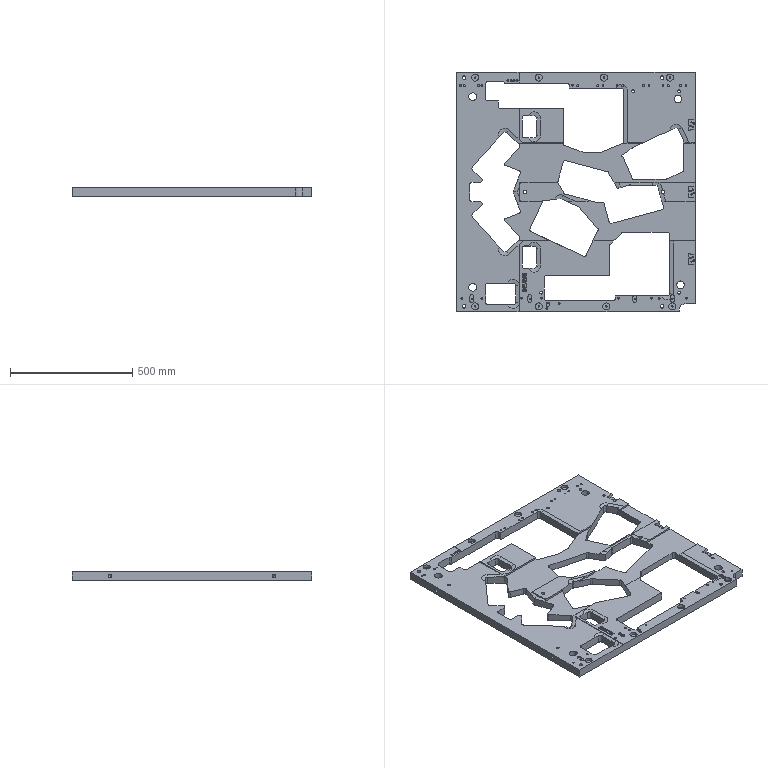Part | NX | features 22 2 | 1 solid | 529 faces | box 975 x 980 x 35 mm | volume 17898134 mm3 | plane 255 | cylinder 184 | cone 64 | spline 26 | commonest cylinder face diameters 20 x41 10 x30 6.8 x22 5.2 x19 6.799 x12 15 x12